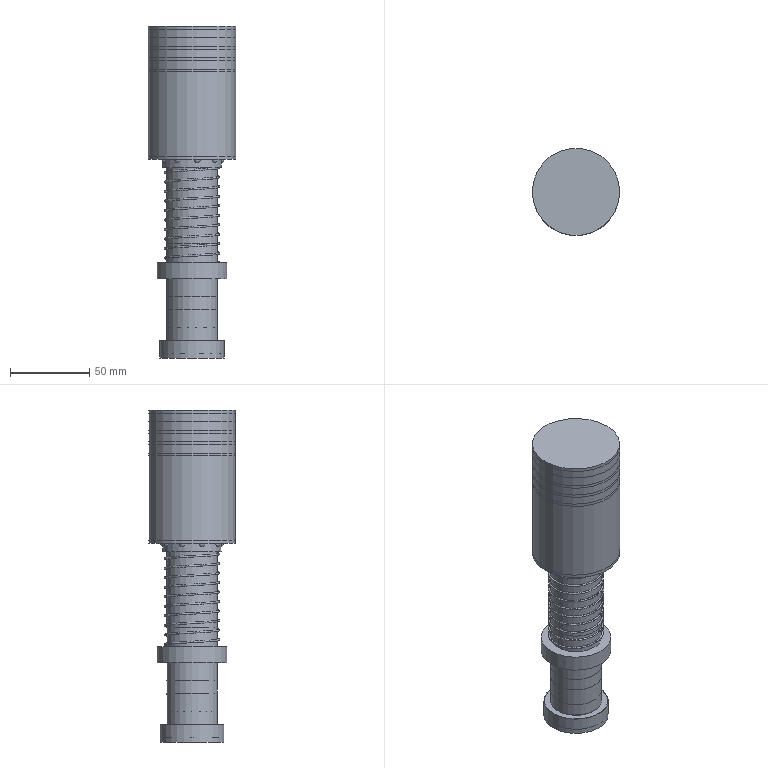Part | NX | features BREP 2 | 11 solids | 252 faces | box 55 x 55 x 209 mm | volume 1026032 mm3 | sphere 162 | plane 43 | cylinder 36 | torus 8 | cone 2 | spline 1 | commonest cylinder face diameters 32 x5 54.996 x4 44 x3 52.246 x3 8 x2 10 x2